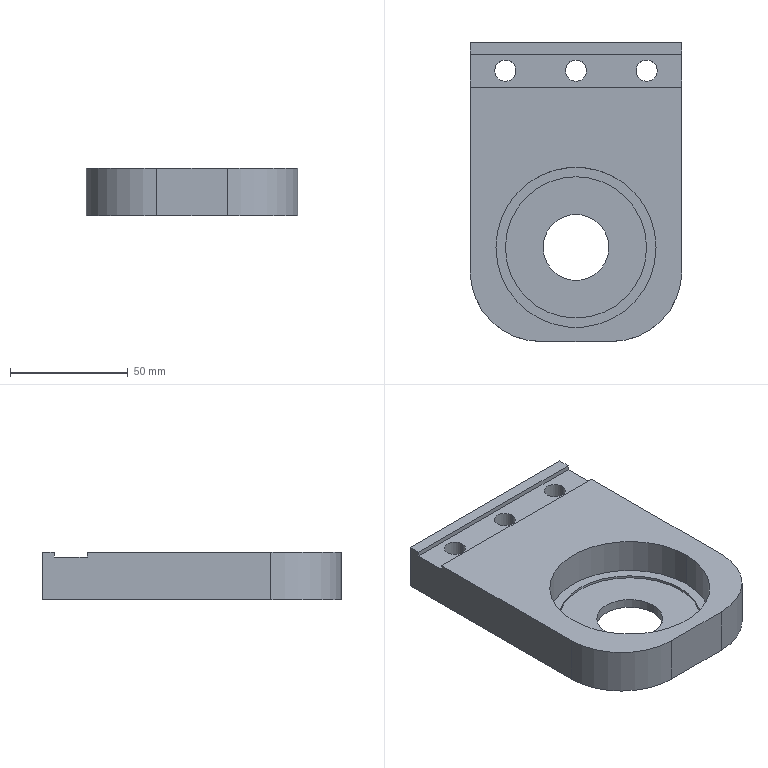Part | SolidWorks | features ICE 4, MoveFace 2, Extrusion 1, Fillet 1, HoleWzd 1 | 1 solid | 35 faces | box 90 x 127.02 x 20 mm | volume 152136 mm3 | cylinder 20 | plane 15 | commonest cylinder face diameters 9 x6 15 x6 60 x4 28 x2 68 x2
STEP:
#1=CARTESIAN_POINT('',(37.5,55.02,9.));
#2=VERTEX_POINT('',#1);
#3=CARTESIAN_POINT('',(22.5,55.02,9.));
#4=VERTEX_POINT('',#3);
#5=CARTESIAN_POINT('',(30.,55.02,9.));
#6=DIRECTION('',(0.,0.,-1.));
#7=DIRECTION('',(-1.,0.,0.));
#8=AXIS2_PLACEMENT_3D('',#5,#6,#7);
#9=CIRCLE('',#8,7.5);
#10=EDGE_CURVE('',#2,#4,#9,.T.);
#11=ORIENTED_EDGE('',*,*,#10,.F.);
#12=CARTESIAN_POINT('',(37.5,55.02,0.));
#13=VERTEX_POINT('',#12);
#14=CARTESIAN_POINT('',(37.5,55.02,0.));
#15=DIRECTION('',(0.,0.,-1.));
#16=VECTOR('',#15,1000.);
#17=LINE('',#14,#16);
#18=EDGE_CURVE('',#2,#13,#17,.T.);
#19=ORIENTED_EDGE('',*,*,#18,.T.);
#20=CARTESIAN_POINT('',(22.5,55.02,0.));
#21=VERTEX_POINT('',#20);
#22=CARTESIAN_POINT('',(30.,55.02,0.));
#23=DIRECTION('',(0.,0.,-1.));
#24=DIRECTION('',(-1.,0.,0.));
#25=AXIS2_PLACEMENT_3D('',#22,#23,#24);
#26=CIRCLE('',#25,7.5);
#27=EDGE_CURVE('',#13,#21,#26,.T.);
#28=ORIENTED_EDGE('',*,*,#27,.T.);
#29=CARTESIAN_POINT('',(22.5,55.02,0.));
#30=DIRECTION('',(0.,0.,-1.));
#31=VECTOR('',#30,1000.);
#32=LINE('',#29,#31);
#33=EDGE_CURVE('',#4,#21,#32,.T.);
#34=ORIENTED_EDGE('',*,*,#33,.F.);
#35=EDGE_LOOP('',(#11,#19,#28,#34));
#36=FACE_OUTER_BOUND('',#35,.T.);
#37=CARTESIAN_POINT('',(30.,55.02,0.));
#38=DIRECTION('',(0.,0.,-1.));
#39=DIRECTION('',(-1.,0.,0.));
#40=AXIS2_PLACEMENT_3D('',#37,#38,#39);
#41=CYLINDRICAL_SURFACE('',#40,7.5);
#42=ADVANCED_FACE('',(#36),#41,.F.);
#43=CARTESIAN_POINT('',(7.5,55.02,9.));
#44=VERTEX_POINT('',#43);
#45=CARTESIAN_POINT('',(-7.5,55.02,9.));
#46=VERTEX_POINT('',#45);
#47=CARTESIAN_POINT('',(0.,55.02,9.));
#48=DIRECTION('',(0.,0.,-1.));
#49=DIRECTION('',(-1.,0.,0.));
#50=AXIS2_PLACEMENT_3D('',#47,#48,#49);
#51=CIRCLE('',#50,7.5);
#52=EDGE_CURVE('',#44,#46,#51,.T.);
#53=ORIENTED_EDGE('',*,*,#52,.F.);
#54=CARTESIAN_POINT('',(7.5,55.02,0.));
#55=VERTEX_POINT('',#54);
#56=CARTESIAN_POINT('',(7.5,55.02,0.));
#57=DIRECTION('',(0.,0.,-1.));
#58=VECTOR('',#57,1000.);
#59=LINE('',#56,#58);
#60=EDGE_CURVE('',#44,#55,#59,.T.);
#61=ORIENTED_EDGE('',*,*,#60,.T.);
#62=CARTESIAN_POINT('',(-7.5,55.02,0.));
#63=VERTEX_POINT('',#62);
#64=CARTESIAN_POINT('',(0.,55.02,0.));
#65=DIRECTION('',(0.,0.,-1.));
#66=DIRECTION('',(-1.,0.,0.));
#67=AXIS2_PLACEMENT_3D('',#64,#65,#66);
#68=CIRCLE('',#67,7.5);
#69=EDGE_CURVE('',#55,#63,#68,.T.);
#70=ORIENTED_EDGE('',*,*,#69,.T.);
#71=CARTESIAN_POINT('',(-7.5,55.02,0.));
#72=DIRECTION('',(0.,0.,-1.));
#73=VECTOR('',#72,1000.);
#74=LINE('',#71,#73);
#75=EDGE_CURVE('',#46,#63,#74,.T.);
#76=ORIENTED_EDGE('',*,*,#75,.F.);
#77=EDGE_LOOP('',(#53,#61,#70,#76));
#78=FACE_OUTER_BOUND('',#77,.T.);
#79=CARTESIAN_POINT('',(0.,55.02,0.));
#80=DIRECTION('',(0.,0.,-1.));
#81=DIRECTION('',(-1.,0.,0.));
#82=AXIS2_PLACEMENT_3D('',#79,#80,#81);
#83=CYLINDRICAL_SURFACE('',#82,7.5);
#84=ADVANCED_FACE('',(#78),#83,.F.);
#85=CARTESIAN_POINT('',(-22.5,55.02,9.));
#86=VERTEX_POINT('',#85);
#87=CARTESIAN_POINT('',(-37.5,55.02,9.));
#88=VERTEX_POINT('',#87);
#89=CARTESIAN_POINT('',(-30.,55.02,9.));
#90=DIRECTION('',(0.,0.,-1.));
#91=DIRECTION('',(-1.,0.,0.));
#92=AXIS2_PLACEMENT_3D('',#89,#90,#91);
#93=CIRCLE('',#92,7.5);
#94=EDGE_CURVE('',#86,#88,#93,.T.);
#95=ORIENTED_EDGE('',*,*,#94,.F.);
#96=CARTESIAN_POINT('',(-22.5,55.02,0.));
#97=VERTEX_POINT('',#96);
#98=CARTESIAN_POINT('',(-22.5,55.02,0.));
#99=DIRECTION('',(0.,0.,-1.));
#100=VECTOR('',#99,1000.);
#101=LINE('',#98,#100);
#102=EDGE_CURVE('',#86,#97,#101,.T.);
#103=ORIENTED_EDGE('',*,*,#102,.T.);
#104=CARTESIAN_POINT('',(-37.5,55.02,0.));
#105=VERTEX_POINT('',#104);
#106=CARTESIAN_POINT('',(-30.,55.02,0.));
#107=DIRECTION('',(0.,0.,-1.));
#108=DIRECTION('',(-1.,0.,0.));
#109=AXIS2_PLACEMENT_3D('',#106,#107,#108);
#110=CIRCLE('',#109,7.5);
#111=EDGE_CURVE('',#97,#105,#110,.T.);
#112=ORIENTED_EDGE('',*,*,#111,.T.);
#113=CARTESIAN_POINT('',(-37.5,55.02,0.));
#114=DIRECTION('',(0.,0.,-1.));
#115=VECTOR('',#114,1000.);
#116=LINE('',#113,#115);
#117=EDGE_CURVE('',#88,#105,#116,.T.);
#118=ORIENTED_EDGE('',*,*,#117,.F.);
#119=EDGE_LOOP('',(#95,#103,#112,#118));
#120=FACE_OUTER_BOUND('',#119,.T.);
#121=CARTESIAN_POINT('',(-30.,55.02,0.));
#122=DIRECTION('',(0.,0.,-1.));
#123=DIRECTION('',(-1.,0.,0.));
#124=AXIS2_PLACEMENT_3D('',#121,#122,#123);
#125=CYLINDRICAL_SURFACE('',#124,7.5);
#126=ADVANCED_FACE('',(#120),#125,.F.);
#127=CARTESIAN_POINT('',(-14.,-20.,0.));
#128=VERTEX_POINT('',#127);
#129=CARTESIAN_POINT('',(14.,-20.,0.));
#130=VERTEX_POINT('',#129);
#131=CARTESIAN_POINT('',(0.,-20.,0.));
#132=DIRECTION('',(0.,0.,1.));
#133=DIRECTION('',(1.,0.,0.));
#134=AXIS2_PLACEMENT_3D('',#131,#132,#133);
#135=CIRCLE('',#134,14.);
#136=EDGE_CURVE('',#128,#130,#135,.T.);
#137=ORIENTED_EDGE('',*,*,#136,.F.);
#138=CARTESIAN_POINT('',(-14.,-20.,4.));
#139=VERTEX_POINT('',#138);
#140=CARTESIAN_POINT('',(-14.,-20.,-6.));
#141=DIRECTION('',(0.,0.,1.));
#142=VECTOR('',#141,1000.);
#143=LINE('',#140,#142);
#144=EDGE_CURVE('',#128,#139,#143,.T.);
#145=ORIENTED_EDGE('',*,*,#144,.T.);
#146=CARTESIAN_POINT('',(14.,-20.,4.));
#147=VERTEX_POINT('',#146);
#148=CARTESIAN_POINT('',(0.,-20.,4.));
#149=DIRECTION('',(0.,0.,1.));
#150=DIRECTION('',(1.,0.,0.));
#151=AXIS2_PLACEMENT_3D('',#148,#149,#150);
#152=CIRCLE('',#151,14.);
#153=EDGE_CURVE('',#139,#147,#152,.T.);
#154=ORIENTED_EDGE('',*,*,#153,.T.);
#155=CARTESIAN_POINT('',(14.,-20.,-6.));
#156=DIRECTION('',(0.,0.,1.));
#157=VECTOR('',#156,1000.);
#158=LINE('',#155,#157);
#159=EDGE_CURVE('',#130,#147,#158,.T.);
#160=ORIENTED_EDGE('',*,*,#159,.F.);
#161=EDGE_LOOP('',(#137,#145,#154,#160));
#162=FACE_OUTER_BOUND('',#161,.T.);
#163=CARTESIAN_POINT('',(0.,-20.,-6.));
#164=DIRECTION('',(0.,0.,1.));
#165=DIRECTION('',(1.,0.,0.));
#166=AXIS2_PLACEMENT_3D('',#163,#164,#165);
#167=CYLINDRICAL_SURFACE('',#166,14.);
#168=ADVANCED_FACE('',(#162),#167,.F.);
#169=CARTESIAN_POINT('',(-30.,-20.,4.));
#170=VERTEX_POINT('',#169);
#171=CARTESIAN_POINT('',(30.,-20.,4.));
#172=VERTEX_POINT('',#171);
#173=CARTESIAN_POINT('',(0.,-20.,4.));
#174=DIRECTION('',(0.,0.,1.));
#175=DIRECTION('',(1.,0.,0.));
#176=AXIS2_PLACEMENT_3D('',#173,#174,#175);
#177=CIRCLE('',#176,30.);
#178=EDGE_CURVE('',#170,#172,#177,.T.);
#179=ORIENTED_EDGE('',*,*,#178,.F.);
#180=CARTESIAN_POINT('',(-30.,-20.,5.));
#181=VERTEX_POINT('',#180);
#182=CARTESIAN_POINT('',(-30.,-20.,4.));
#183=DIRECTION('',(0.,0.,1.));
#184=VECTOR('',#183,1000.);
#185=LINE('',#182,#184);
#186=EDGE_CURVE('',#170,#181,#185,.T.);
#187=ORIENTED_EDGE('',*,*,#186,.T.);
#188=CARTESIAN_POINT('',(30.,-20.,5.));
#189=VERTEX_POINT('',#188);
#190=CARTESIAN_POINT('',(0.,-20.,5.));
#191=DIRECTION('',(0.,0.,1.));
#192=DIRECTION('',(1.,0.,0.));
#193=AXIS2_PLACEMENT_3D('',#190,#191,#192);
#194=CIRCLE('',#193,30.);
#195=EDGE_CURVE('',#181,#189,#194,.T.);
#196=ORIENTED_EDGE('',*,*,#195,.T.);
#197=CARTESIAN_POINT('',(30.,-20.,4.));
#198=DIRECTION('',(0.,0.,1.));
#199=VECTOR('',#198,1000.);
#200=LINE('',#197,#199);
#201=EDGE_CURVE('',#172,#189,#200,.T.);
#202=ORIENTED_EDGE('',*,*,#201,.F.);
#203=EDGE_LOOP('',(#179,#187,#196,#202));
#204=FACE_OUTER_BOUND('',#203,.T.);
#205=CARTESIAN_POINT('',(0.,-20.,4.));
#206=DIRECTION('',(0.,0.,1.));
#207=DIRECTION('',(1.,0.,0.));
#208=AXIS2_PLACEMENT_3D('',#205,#206,#207);
#209=CYLINDRICAL_SURFACE('',#208,30.);
#210=ADVANCED_FACE('',(#204),#209,.F.);
#211=CARTESIAN_POINT('',(-34.,-20.,5.));
#212=VERTEX_POINT('',#211);
#213=CARTESIAN_POINT('',(34.,-20.,5.));
#214=VERTEX_POINT('',#213);
#215=CARTESIAN_POINT('',(0.,-20.,5.));
#216=DIRECTION('',(0.,0.,1.));
#217=DIRECTION('',(1.,0.,0.));
#218=AXIS2_PLACEMENT_3D('',#215,#216,#217);
#219=CIRCLE('',#218,34.);
#220=EDGE_CURVE('',#212,#214,#219,.T.);
#221=ORIENTED_EDGE('',*,*,#220,.F.);
#222=CARTESIAN_POINT('',(-34.,-20.,20.));
#223=VERTEX_POINT('',#222);
#224=CARTESIAN_POINT('',(-34.,-20.,5.));
#225=DIRECTION('',(0.,0.,1.));
#226=VECTOR('',#225,1000.);
#227=LINE('',#224,#226);
#228=EDGE_CURVE('',#212,#223,#227,.T.);
#229=ORIENTED_EDGE('',*,*,#228,.T.);
#230=CARTESIAN_POINT('',(34.,-20.,20.));
#231=VERTEX_POINT('',#230);
#232=CARTESIAN_POINT('',(0.,-20.,20.));
#233=DIRECTION('',(0.,0.,1.));
#234=DIRECTION('',(1.,0.,0.));
#235=AXIS2_PLACEMENT_3D('',#232,#233,#234);
#236=CIRCLE('',#235,34.);
#237=EDGE_CURVE('',#223,#231,#236,.T.);
#238=ORIENTED_EDGE('',*,*,#237,.T.);
#239=CARTESIAN_POINT('',(34.,-20.,5.));
#240=DIRECTION('',(0.,0.,1.));
#241=VECTOR('',#240,1000.);
#242=LINE('',#239,#241);
#243=EDGE_CURVE('',#214,#231,#242,.T.);
#244=ORIENTED_EDGE('',*,*,#243,.F.);
#245=EDGE_LOOP('',(#221,#229,#238,#244));
#246=FACE_OUTER_BOUND('',#245,.T.);
#247=CARTESIAN_POINT('',(0.,-20.,5.));
#248=DIRECTION('',(0.,0.,1.));
#249=DIRECTION('',(1.,0.,0.));
#250=AXIS2_PLACEMENT_3D('',#247,#248,#249);
#251=CYLINDRICAL_SURFACE('',#250,34.);
#252=ADVANCED_FACE('',(#246),#251,.F.);
#253=CARTESIAN_POINT('',(34.5,55.02,18.));
#254=VERTEX_POINT('',#253);
#255=CARTESIAN_POINT('',(25.5,55.02,18.));
#256=VERTEX_POINT('',#255);
#257=CARTESIAN_POINT('',(30.,55.02,18.));
#258=DIRECTION('',(0.,0.,-1.));
#259=DIRECTION('',(1.,0.,0.));
#260=AXIS2_PLACEMENT_3D('',#257,#258,#259);
#261=CIRCLE('',#260,4.5);
#262=EDGE_CURVE('',#254,#256,#261,.T.);
#263=ORIENTED_EDGE('',*,*,#262,.F.);
#264=CARTESIAN_POINT('',(34.5,55.02,9.));
#265=VERTEX_POINT('',#264);
#266=CARTESIAN_POINT('',(34.5,55.02,0.));
#267=DIRECTION('',(0.,0.,-1.));
#268=VECTOR('',#267,1000.);
#269=LINE('',#266,#268);
#270=EDGE_CURVE('',#254,#265,#269,.T.);
#271=ORIENTED_EDGE('',*,*,#270,.T.);
#272=CARTESIAN_POINT('',(25.5,55.02,9.));
#273=VERTEX_POINT('',#272);
#274=CARTESIAN_POINT('',(30.,55.02,9.));
#275=DIRECTION('',(0.,0.,-1.));
#276=DIRECTION('',(-1.,0.,0.));
#277=AXIS2_PLACEMENT_3D('',#274,#275,#276);
#278=CIRCLE('',#277,4.5);
#279=EDGE_CURVE('',#265,#273,#278,.T.);
#280=ORIENTED_EDGE('',*,*,#279,.T.);
#281=CARTESIAN_POINT('',(25.5,55.02,0.));
#282=DIRECTION('',(0.,0.,-1.));
#283=VECTOR('',#282,1000.);
#284=LINE('',#281,#283);
#285=EDGE_CURVE('',#256,#273,#284,.T.);
#286=ORIENTED_EDGE('',*,*,#285,.F.);
#287=EDGE_LOOP('',(#263,#271,#280,#286));
#288=FACE_OUTER_BOUND('',#287,.T.);
#289=CARTESIAN_POINT('',(30.,55.02,0.));
#290=DIRECTION('',(0.,0.,-1.));
#291=DIRECTION('',(-1.,0.,0.));
#292=AXIS2_PLACEMENT_3D('',#289,#290,#291);
#293=CYLINDRICAL_SURFACE('',#292,4.5);
#294=ADVANCED_FACE('',(#288),#293,.F.);
#295=CARTESIAN_POINT('',(4.5,55.02,18.));
#296=VERTEX_POINT('',#295);
#297=CARTESIAN_POINT('',(-4.5,55.02,18.));
#298=VERTEX_POINT('',#297);
#299=CARTESIAN_POINT('',(0.,55.02,18.));
#300=DIRECTION('',(0.,0.,-1.));
#301=DIRECTION('',(1.,0.,0.));
#302=AXIS2_PLACEMENT_3D('',#299,#300,#301);
#303=CIRCLE('',#302,4.5);
#304=EDGE_CURVE('',#296,#298,#303,.T.);
#305=ORIENTED_EDGE('',*,*,#304,.F.);
#306=CARTESIAN_POINT('',(4.5,55.02,9.));
#307=VERTEX_POINT('',#306);
#308=CARTESIAN_POINT('',(4.5,55.02,0.));
#309=DIRECTION('',(0.,0.,-1.));
#310=VECTOR('',#309,1000.);
#311=LINE('',#308,#310);
#312=EDGE_CURVE('',#296,#307,#311,.T.);
#313=ORIENTED_EDGE('',*,*,#312,.T.);
#314=CARTESIAN_POINT('',(-4.5,55.02,9.));
#315=VERTEX_POINT('',#314);
#316=CARTESIAN_POINT('',(0.,55.02,9.));
#317=DIRECTION('',(0.,0.,-1.));
#318=DIRECTION('',(-1.,0.,0.));
#319=AXIS2_PLACEMENT_3D('',#316,#317,#318);
#320=CIRCLE('',#319,4.5);
#321=EDGE_CURVE('',#307,#315,#320,.T.);
#322=ORIENTED_EDGE('',*,*,#321,.T.);
#323=CARTESIAN_POINT('',(-4.5,55.02,0.));
#324=DIRECTION('',(0.,0.,-1.));
#325=VECTOR('',#324,1000.);
#326=LINE('',#323,#325);
#327=EDGE_CURVE('',#298,#315,#326,.T.);
#328=ORIENTED_EDGE('',*,*,#327,.F.);
#329=EDGE_LOOP('',(#305,#313,#322,#328));
#330=FACE_OUTER_BOUND('',#329,.T.);
#331=CARTESIAN_POINT('',(0.,55.02,0.));
#332=DIRECTION('',(0.,0.,-1.));
#333=DIRECTION('',(-1.,0.,0.));
#334=AXIS2_PLACEMENT_3D('',#331,#332,#333);
#335=CYLINDRICAL_SURFACE('',#334,4.5);
#336=ADVANCED_FACE('',(#330),#335,.F.);
#337=CARTESIAN_POINT('',(-25.5,55.02,18.));
#338=VERTEX_POINT('',#337);
#339=CARTESIAN_POINT('',(-34.5,55.02,18.));
#340=VERTEX_POINT('',#339);
#341=CARTESIAN_POINT('',(-30.,55.02,18.));
#342=DIRECTION('',(0.,0.,-1.));
#343=DIRECTION('',(1.,0.,0.));
#344=AXIS2_PLACEMENT_3D('',#341,#342,#343);
#345=CIRCLE('',#344,4.5);
#346=EDGE_CURVE('',#338,#340,#345,.T.);
#347=ORIENTED_EDGE('',*,*,#346,.F.);
#348=CARTESIAN_POINT('',(-25.5,55.02,9.));
#349=VERTEX_POINT('',#348);
#350=CARTESIAN_POINT('',(-25.5,55.02,0.));
#351=DIRECTION('',(0.,0.,-1.));
#352=VECTOR('',#351,1000.);
#353=LINE('',#350,#352);
#354=EDGE_CURVE('',#338,#349,#353,.T.);
#355=ORIENTED_EDGE('',*,*,#354,.T.);
#356=CARTESIAN_POINT('',(-34.5,55.02,9.));
#357=VERTEX_POINT('',#356);
#358=CARTESIAN_POINT('',(-30.,55.02,9.));
#359=DIRECTION('',(0.,0.,-1.));
#360=DIRECTION('',(-1.,0.,0.));
#361=AXIS2_PLACEMENT_3D('',#358,#359,#360);
#362=CIRCLE('',#361,4.5);
#363=EDGE_CURVE('',#349,#357,#362,.T.);
#364=ORIENTED_EDGE('',*,*,#363,.T.);
#365=CARTESIAN_POINT('',(-34.5,55.02,0.));
#366=DIRECTION('',(0.,0.,-1.));
#367=VECTOR('',#366,1000.);
#368=LINE('',#365,#367);
#369=EDGE_CURVE('',#340,#357,#368,.T.);
#370=ORIENTED_EDGE('',*,*,#369,.F.);
#371=EDGE_LOOP('',(#347,#355,#364,#370));
#372=FACE_OUTER_BOUND('',#371,.T.);
#373=CARTESIAN_POINT('',(-30.,55.02,0.));
#374=DIRECTION('',(0.,0.,-1.));
#375=DIRECTION('',(-1.,0.,0.));
#376=AXIS2_PLACEMENT_3D('',#373,#374,#375);
#377=CYLINDRICAL_SURFACE('',#376,4.5);
#378=ADVANCED_FACE('',(#372),#377,.F.);
#379=CARTESIAN_POINT('',(45.,62.02,20.));
#380=VERTEX_POINT('',#379);
#381=CARTESIAN_POINT('',(-45.,62.02,20.));
#382=VERTEX_POINT('',#381);
#383=CARTESIAN_POINT('',(-45.,62.02,20.));
#384=DIRECTION('',(-1.,0.,0.));
#385=VECTOR('',#384,1000.);
#386=LINE('',#383,#385);
#387=EDGE_CURVE('',#380,#382,#386,.T.);
#388=ORIENTED_EDGE('',*,*,#387,.F.);
#389=CARTESIAN_POINT('',(45.,67.02,20.));
#390=VERTEX_POINT('',#389);
#391=CARTESIAN_POINT('',(45.,60.,20.));
#392=DIRECTION('',(0.,1.,0.));
#393=VECTOR('',#392,1000.);
#394=LINE('',#391,#393);
#395=EDGE_CURVE('',#380,#390,#394,.T.);
#396=ORIENTED_EDGE('',*,*,#395,.T.);
#397=CARTESIAN_POINT('',(-45.,67.02,20.));
#398=VERTEX_POINT('',#397);
#399=CARTESIAN_POINT('',(-45.,67.02,20.));
#400=DIRECTION('',(-1.,0.,0.));
#401=VECTOR('',#400,1000.);
#402=LINE('',#399,#401);
#403=EDGE_CURVE('',#390,#398,#402,.T.);
#404=ORIENTED_EDGE('',*,*,#403,.T.);
#405=CARTESIAN_POINT('',(-45.,60.,20.));
#406=DIRECTION('',(0.,-1.,0.));
#407=VECTOR('',#406,1000.);
#408=LINE('',#405,#407);
#409=EDGE_CURVE('',#398,#382,#408,.T.);
#410=ORIENTED_EDGE('',*,*,#409,.T.);
#411=EDGE_LOOP('',(#388,#396,#404,#410));
#412=FACE_OUTER_BOUND('',#411,.T.);
#413=CARTESIAN_POINT('',(0.,0.,20.));
#414=DIRECTION('',(0.,0.,1.));
#415=DIRECTION('',(1.,0.,0.));
#416=AXIS2_PLACEMENT_3D('',#413,#414,#415);
#417=PLANE('',#416);
#418=ADVANCED_FACE('',(#412),#417,.T.);
#419=ORIENTED_EDGE('',*,*,#354,.F.);
#420=CARTESIAN_POINT('',(-30.,55.02,18.));
#421=DIRECTION('',(0.,0.,-1.));
#422=DIRECTION('',(1.,0.,0.));
#423=AXIS2_PLACEMENT_3D('',#420,#421,#422);
#424=CIRCLE('',#423,4.5);
#425=EDGE_CURVE('',#340,#338,#424,.T.);
#426=ORIENTED_EDGE('',*,*,#425,.F.);
#427=ORIENTED_EDGE('',*,*,#369,.T.);
#428=CARTESIAN_POINT('',(-30.,55.02,9.));
#429=DIRECTION('',(0.,0.,-1.));
#430=DIRECTION('',(-1.,0.,0.));
#431=AXIS2_PLACEMENT_3D('',#428,#429,#430);
#432=CIRCLE('',#431,4.5);
#433=EDGE_CURVE('',#357,#349,#432,.T.);
#434=ORIENTED_EDGE('',*,*,#433,.T.);
#435=EDGE_LOOP('',(#419,#426,#427,#434));
#436=FACE_OUTER_BOUND('',#435,.T.);
#437=CARTESIAN_POINT('',(-30.,55.02,0.));
#438=DIRECTION('',(0.,0.,-1.));
#439=DIRECTION('',(-1.,0.,0.));
#440=AXIS2_PLACEMENT_3D('',#437,#438,#439);
#441=CYLINDRICAL_SURFACE('',#440,4.5);
#442=ADVANCED_FACE('',(#436),#441,.F.);
#443=ORIENTED_EDGE('',*,*,#312,.F.);
#444=CARTESIAN_POINT('',(0.,55.02,18.));
#445=DIRECTION('',(0.,0.,-1.));
#446=DIRECTION('',(1.,0.,0.));
#447=AXIS2_PLACEMENT_3D('',#444,#445,#446);
#448=CIRCLE('',#447,4.5);
#449=EDGE_CURVE('',#298,#296,#448,.T.);
#450=ORIENTED_EDGE('',*,*,#449,.F.);
#451=ORIENTED_EDGE('',*,*,#327,.T.);
#452=CARTESIAN_POINT('',(0.,55.02,9.));
#453=DIRECTION('',(0.,0.,-1.));
#454=DIRECTION('',(-1.,0.,0.));
#455=AXIS2_PLACEMENT_3D('',#452,#453,#454);
#456=CIRCLE('',#455,4.5);
#457=EDGE_CURVE('',#315,#307,#456,.T.);
#458=ORIENTED_EDGE('',*,*,#457,.T.);
#459=EDGE_LOOP('',(#443,#450,#451,#458));
#460=FACE_OUTER_BOUND('',#459,.T.);
#461=CARTESIAN_POINT('',(0.,55.02,0.));
#462=DIRECTION('',(0.,0.,-1.));
#463=DIRECTION('',(-1.,0.,0.));
#464=AXIS2_PLACEMENT_3D('',#461,#462,#463);
#465=CYLINDRICAL_SURFACE('',#464,4.5);
#466=ADVANCED_FACE('',(#460),#465,.F.);
#467=ORIENTED_EDGE('',*,*,#270,.F.);
#468=CARTESIAN_POINT('',(30.,55.02,18.));
#469=DIRECTION('',(0.,0.,-1.));
#470=DIRECTION('',(1.,0.,0.));
#471=AXIS2_PLACEMENT_3D('',#468,#469,#470);
#472=CIRCLE('',#471,4.5);
#473=EDGE_CURVE('',#256,#254,#472,.T.);
#474=ORIENTED_EDGE('',*,*,#473,.F.);
#475=ORIENTED_EDGE('',*,*,#285,.T.);
#476=CARTESIAN_POINT('',(30.,55.02,9.));
#477=DIRECTION('',(0.,0.,-1.));
#478=DIRECTION('',(-1.,0.,0.));
#479=AXIS2_PLACEMENT_3D('',#476,#477,#478);
#480=CIRCLE('',#479,4.5);
#481=EDGE_CURVE('',#273,#265,#480,.T.);
#482=ORIENTED_EDGE('',*,*,#481,.T.);
#483=EDGE_LOOP('',(#467,#474,#475,#482));
#484=FACE_OUTER_BOUND('',#483,.T.);
#485=CARTESIAN_POINT('',(30.,55.02,0.));
#486=DIRECTION('',(0.,0.,-1.));
#487=DIRECTION('',(-1.,0.,0.));
#488=AXIS2_PLACEMENT_3D('',#485,#486,#487);
#489=CYLINDRICAL_SURFACE('',#488,4.5);
#490=ADVANCED_FACE('',(#484),#489,.F.);
#491=ORIENTED_EDGE('',*,*,#395,.F.);
#492=CARTESIAN_POINT('',(45.,62.02,18.));
#493=VERTEX_POINT('',#492);
#494=CARTESIAN_POINT('',(45.,62.02,18.));
#495=DIRECTION('',(0.,0.,1.));
#496=VECTOR('',#495,1000.);
#497=LINE('',#494,#496);
#498=EDGE_CURVE('',#493,#380,#497,.T.);
#499=ORIENTED_EDGE('',*,*,#498,.F.);
#500=CARTESIAN_POINT('',(45.,48.02,18.));
#501=VERTEX_POINT('',#500);
#502=CARTESIAN_POINT('',(45.,62.02,18.));
#503=DIRECTION('',(0.,1.,0.));
#504=VECTOR('',#503,1000.);
#505=LINE('',#502,#504);
#506=EDGE_CURVE('',#501,#493,#505,.T.);
#507=ORIENTED_EDGE('',*,*,#506,.F.);
#508=CARTESIAN_POINT('',(45.,48.02,20.));
#509=VERTEX_POINT('',#508);
#510=CARTESIAN_POINT('',(45.,48.02,18.));
#511=DIRECTION('',(0.,0.,1.));
#512=VECTOR('',#511,1000.);
#513=LINE('',#510,#512);
#514=EDGE_CURVE('',#501,#509,#513,.T.);
#515=ORIENTED_EDGE('',*,*,#514,.T.);
#516=CARTESIAN_POINT('',(45.,-30.,20.));
#517=VERTEX_POINT('',#516);
#518=CARTESIAN_POINT('',(45.,60.,20.));
#519=DIRECTION('',(0.,1.,0.));
#520=VECTOR('',#519,1000.);
#521=LINE('',#518,#520);
#522=EDGE_CURVE('',#517,#509,#521,.T.);
#523=ORIENTED_EDGE('',*,*,#522,.F.);
#524=CARTESIAN_POINT('',(45.,-30.,0.));
#525=VERTEX_POINT('',#524);
#526=CARTESIAN_POINT('',(45.,-30.,20.));
#527=DIRECTION('',(0.,0.,-1.));
#528=VECTOR('',#527,1000.);
#529=LINE('',#526,#528);
#530=EDGE_CURVE('',#517,#525,#529,.T.);
#531=ORIENTED_EDGE('',*,*,#530,.T.);
#532=CARTESIAN_POINT('',(45.,67.02,0.));
#533=VERTEX_POINT('',#532);
#534=CARTESIAN_POINT('',(45.,60.,0.));
#535=DIRECTION('',(0.,1.,0.));
#536=VECTOR('',#535,1000.);
#537=LINE('',#534,#536);
#538=EDGE_CURVE('',#525,#533,#537,.T.);
#539=ORIENTED_EDGE('',*,*,#538,.T.);
#540=CARTESIAN_POINT('',(45.,67.02,20.));
#541=DIRECTION('',(0.,0.,-1.));
#542=VECTOR('',#541,1000.);
#543=LINE('',#540,#542);
#544=EDGE_CURVE('',#390,#533,#543,.T.);
#545=ORIENTED_EDGE('',*,*,#544,.F.);
#546=EDGE_LOOP('',(#491,#499,#507,#515,#523,#531,#539,#545));
#547=FACE_OUTER_BOUND('',#546,.T.);
#548=CARTESIAN_POINT('',(45.,60.,20.));
#549=DIRECTION('',(-1.,0.,0.));
#550=DIRECTION('',(0.,-1.,0.));
#551=AXIS2_PLACEMENT_3D('',#548,#549,#550);
#552=PLANE('',#551);
#553=ADVANCED_FACE('',(#547),#552,.F.);
#554=CARTESIAN_POINT('',(-45.,67.02,0.));
#555=VERTEX_POINT('',#554);
#556=CARTESIAN_POINT('',(-45.,67.02,0.));
#557=DIRECTION('',(-1.,0.,0.));
#558=VECTOR('',#557,1000.);
#559=LINE('',#556,#558);
#560=EDGE_CURVE('',#533,#555,#559,.T.);
#561=ORIENTED_EDGE('',*,*,#560,.T.);
#562=CARTESIAN_POINT('',(-45.,67.02,20.));
#563=DIRECTION('',(0.,0.,-1.));
#564=VECTOR('',#563,1000.);
#565=LINE('',#562,#564);
#566=EDGE_CURVE('',#398,#555,#565,.T.);
#567=ORIENTED_EDGE('',*,*,#566,.F.);
#568=ORIENTED_EDGE('',*,*,#403,.F.);
#569=ORIENTED_EDGE('',*,*,#544,.T.);
#570=EDGE_LOOP('',(#561,#567,#568,#569));
#571=FACE_OUTER_BOUND('',#570,.T.);
#572=CARTESIAN_POINT('',(-45.,67.02,20.));
#573=DIRECTION('',(0.,-1.,0.));
#574=DIRECTION('',(0.,0.,-1.));
#575=AXIS2_PLACEMENT_3D('',#572,#573,#574);
#576=PLANE('',#575);
#577=ADVANCED_FACE('',(#571),#576,.F.);
#578=CARTESIAN_POINT('',(-45.,62.02,18.));
#579=VERTEX_POINT('',#578);
#580=CARTESIAN_POINT('',(-45.,48.02,18.));
#581=VERTEX_POINT('',#580);
#582=CARTESIAN_POINT('',(-45.,62.02,18.));
#583=DIRECTION('',(0.,-1.,0.));
#584=VECTOR('',#583,1000.);
#585=LINE('',#582,#584);
#586=EDGE_CURVE('',#579,#581,#585,.T.);
#587=ORIENTED_EDGE('',*,*,#586,.F.);
#588=CARTESIAN_POINT('',(-45.,62.02,18.));
#589=DIRECTION('',(0.,0.,1.));
#590=VECTOR('',#589,1000.);
#591=LINE('',#588,#590);
#592=EDGE_CURVE('',#579,#382,#591,.T.);
#593=ORIENTED_EDGE('',*,*,#592,.T.);
#594=ORIENTED_EDGE('',*,*,#409,.F.);
#595=ORIENTED_EDGE('',*,*,#566,.T.);
#596=CARTESIAN_POINT('',(-45.,-30.,0.));
#597=VERTEX_POINT('',#596);
#598=CARTESIAN_POINT('',(-45.,60.,0.));
#599=DIRECTION('',(0.,-1.,0.));
#600=VECTOR('',#599,1000.);
#601=LINE('',#598,#600);
#602=EDGE_CURVE('',#555,#597,#601,.T.);
#603=ORIENTED_EDGE('',*,*,#602,.T.);
#604=CARTESIAN_POINT('',(-45.,-30.,20.));
#605=VERTEX_POINT('',#604);
#606=CARTESIAN_POINT('',(-45.,-30.,20.));
#607=DIRECTION('',(0.,0.,1.));
#608=VECTOR('',#607,1000.);
#609=LINE('',#606,#608);
#610=EDGE_CURVE('',#597,#605,#609,.T.);
#611=ORIENTED_EDGE('',*,*,#610,.T.);
#612=CARTESIAN_POINT('',(-45.,48.02,20.));
#613=VERTEX_POINT('',#612);
#614=CARTESIAN_POINT('',(-45.,60.,20.));
#615=DIRECTION('',(0.,-1.,0.));
#616=VECTOR('',#615,1000.);
#617=LINE('',#614,#616);
#618=EDGE_CURVE('',#613,#605,#617,.T.);
#619=ORIENTED_EDGE('',*,*,#618,.F.);
#620=CARTESIAN_POINT('',(-45.,48.02,18.));
#621=DIRECTION('',(0.,0.,1.));
#622=VECTOR('',#621,1000.);
#623=LINE('',#620,#622);
#624=EDGE_CURVE('',#581,#613,#623,.T.);
#625=ORIENTED_EDGE('',*,*,#624,.F.);
#626=EDGE_LOOP('',(#587,#593,#594,#595,#603,#611,#619,#625));
#627=FACE_OUTER_BOUND('',#626,.T.);
#628=CARTESIAN_POINT('',(-45.,60.,20.));
#629=DIRECTION('',(1.,0.,0.));
#630=DIRECTION('',(0.,1.,0.));
#631=AXIS2_PLACEMENT_3D('',#628,#629,#630);
#632=PLANE('',#631);
#633=ADVANCED_FACE('',(#627),#632,.F.);
#634=CARTESIAN_POINT('',(-15.,-60.,0.));
#635=VERTEX_POINT('',#634);
#636=CARTESIAN_POINT('',(15.,-60.,0.));
#637=VERTEX_POINT('',#636);
#638=CARTESIAN_POINT('',(-45.,-60.,0.));
#639=DIRECTION('',(1.,0.,0.));
#640=VECTOR('',#639,1000.);
#641=LINE('',#638,#640);
#642=EDGE_CURVE('',#635,#637,#641,.T.);
#643=ORIENTED_EDGE('',*,*,#642,.T.);
#644=CARTESIAN_POINT('',(15.,-60.,20.));
#645=VERTEX_POINT('',#644);
#646=CARTESIAN_POINT('',(15.,-60.,20.));
#647=DIRECTION('',(0.,0.,1.));
#648=VECTOR('',#647,1000.);
#649=LINE('',#646,#648);
#650=EDGE_CURVE('',#637,#645,#649,.T.);
#651=ORIENTED_EDGE('',*,*,#650,.T.);
#652=CARTESIAN_POINT('',(-15.,-60.,20.));
#653=VERTEX_POINT('',#652);
#654=CARTESIAN_POINT('',(-45.,-60.,20.));
#655=DIRECTION('',(1.,0.,0.));
#656=VECTOR('',#655,1000.);
#657=LINE('',#654,#656);
#658=EDGE_CURVE('',#653,#645,#657,.T.);
#659=ORIENTED_EDGE('',*,*,#658,.F.);
#660=CARTESIAN_POINT('',(-15.,-60.,20.));
#661=DIRECTION('',(0.,0.,-1.));
#662=VECTOR('',#661,1000.);
#663=LINE('',#660,#662);
#664=EDGE_CURVE('',#653,#635,#663,.T.);
#665=ORIENTED_EDGE('',*,*,#664,.T.);
#666=EDGE_LOOP('',(#643,#651,#659,#665));
#667=FACE_OUTER_BOUND('',#666,.T.);
#668=CARTESIAN_POINT('',(-45.,-60.,20.));
#669=DIRECTION('',(0.,1.,0.));
#670=DIRECTION('',(0.,0.,1.));
#671=AXIS2_PLACEMENT_3D('',#668,#669,#670);
#672=PLANE('',#671);
#673=ADVANCED_FACE('',(#667),#672,.F.);
#674=CARTESIAN_POINT('',(-45.,48.02,20.));
#675=DIRECTION('',(1.,0.,0.));
#676=VECTOR('',#675,1000.);
#677=LINE('',#674,#676);
#678=EDGE_CURVE('',#613,#509,#677,.T.);
#679=ORIENTED_EDGE('',*,*,#678,.F.);
#680=ORIENTED_EDGE('',*,*,#618,.T.);
#681=CARTESIAN_POINT('',(-15.,-30.,20.));
#682=DIRECTION('',(0.,0.,1.));
#683=DIRECTION('',(1.,0.,0.));
#684=AXIS2_PLACEMENT_3D('',#681,#682,#683);
#685=CIRCLE('',#684,30.);
#686=EDGE_CURVE('',#605,#653,#685,.T.);
#687=ORIENTED_EDGE('',*,*,#686,.T.);
#688=ORIENTED_EDGE('',*,*,#658,.T.);
#689=CARTESIAN_POINT('',(15.,-30.,20.));
#690=DIRECTION('',(0.,0.,1.));
#691=DIRECTION('',(1.,0.,0.));
#692=AXIS2_PLACEMENT_3D('',#689,#690,#691);
#693=CIRCLE('',#692,30.);
#694=EDGE_CURVE('',#645,#517,#693,.T.);
#695=ORIENTED_EDGE('',*,*,#694,.T.);
#696=ORIENTED_EDGE('',*,*,#522,.T.);
#697=EDGE_LOOP('',(#679,#680,#687,#688,#695,#696));
#698=FACE_OUTER_BOUND('',#697,.T.);
#699=CARTESIAN_POINT('',(0.,-20.,20.));
#700=DIRECTION('',(0.,0.,1.));
#701=DIRECTION('',(1.,0.,0.));
#702=AXIS2_PLACEMENT_3D('',#699,#700,#701);
#703=CIRCLE('',#702,34.);
#704=EDGE_CURVE('',#231,#223,#703,.T.);
#705=ORIENTED_EDGE('',*,*,#704,.F.);
#706=ORIENTED_EDGE('',*,*,#237,.F.);
#707=EDGE_LOOP('',(#705,#706));
#708=FACE_BOUND('',#707,.T.);
#709=CARTESIAN_POINT('',(0.,0.,20.));
#710=DIRECTION('',(0.,0.,1.));
#711=DIRECTION('',(1.,0.,0.));
#712=AXIS2_PLACEMENT_3D('',#709,#710,#711);
#713=PLANE('',#712);
#714=ADVANCED_FACE('',(#698,#708),#713,.T.);
#715=CARTESIAN_POINT('',(30.,55.02,0.));
#716=DIRECTION('',(0.,0.,-1.));
#717=DIRECTION('',(-1.,0.,0.));
#718=AXIS2_PLACEMENT_3D('',#715,#716,#717);
#719=CIRCLE('',#718,7.5);
#720=EDGE_CURVE('',#21,#13,#719,.T.);
#721=ORIENTED_EDGE('',*,*,#720,.F.);
#722=ORIENTED_EDGE('',*,*,#27,.F.);
#723=EDGE_LOOP('',(#721,#722));
#724=FACE_BOUND('',#723,.T.);
#725=CARTESIAN_POINT('',(0.,55.02,0.));
#726=DIRECTION('',(0.,0.,-1.));
#727=DIRECTION('',(-1.,0.,0.));
#728=AXIS2_PLACEMENT_3D('',#725,#726,#727);
#729=CIRCLE('',#728,7.5);
#730=EDGE_CURVE('',#63,#55,#729,.T.);
#731=ORIENTED_EDGE('',*,*,#730,.F.);
#732=ORIENTED_EDGE('',*,*,#69,.F.);
#733=EDGE_LOOP('',(#731,#732));
#734=FACE_BOUND('',#733,.T.);
#735=CARTESIAN_POINT('',(-30.,55.02,0.));
#736=DIRECTION('',(0.,0.,-1.));
#737=DIRECTION('',(-1.,0.,0.));
#738=AXIS2_PLACEMENT_3D('',#735,#736,#737);
#739=CIRCLE('',#738,7.5);
#740=EDGE_CURVE('',#105,#97,#739,.T.);
#741=ORIENTED_EDGE('',*,*,#740,.F.);
#742=ORIENTED_EDGE('',*,*,#111,.F.);
#743=EDGE_LOOP('',(#741,#742));
#744=FACE_BOUND('',#743,.T.);
#745=CARTESIAN_POINT('',(0.,-20.,0.));
#746=DIRECTION('',(0.,0.,1.));
#747=DIRECTION('',(1.,0.,0.));
#748=AXIS2_PLACEMENT_3D('',#745,#746,#747);
#749=CIRCLE('',#748,14.);
#750=EDGE_CURVE('',#130,#128,#749,.T.);
#751=ORIENTED_EDGE('',*,*,#750,.T.);
#752=ORIENTED_EDGE('',*,*,#136,.T.);
#753=EDGE_LOOP('',(#751,#752));
#754=FACE_BOUND('',#753,.T.);
#755=ORIENTED_EDGE('',*,*,#538,.F.);
#756=CARTESIAN_POINT('',(15.,-30.,0.));
#757=DIRECTION('',(0.,0.,-1.));
#758=DIRECTION('',(1.,0.,0.));
#759=AXIS2_PLACEMENT_3D('',#756,#757,#758);
#760=CIRCLE('',#759,30.);
#761=EDGE_CURVE('',#525,#637,#760,.T.);
#762=ORIENTED_EDGE('',*,*,#761,.T.);
#763=ORIENTED_EDGE('',*,*,#642,.F.);
#764=CARTESIAN_POINT('',(-15.,-30.,0.));
#765=DIRECTION('',(0.,0.,-1.));
#766=DIRECTION('',(1.,0.,0.));
#767=AXIS2_PLACEMENT_3D('',#764,#765,#766);
#768=CIRCLE('',#767,30.);
#769=EDGE_CURVE('',#635,#597,#768,.T.);
#770=ORIENTED_EDGE('',*,*,#769,.T.);
#771=ORIENTED_EDGE('',*,*,#602,.F.);
#772=ORIENTED_EDGE('',*,*,#560,.F.);
#773=EDGE_LOOP('',(#755,#762,#763,#770,#771,#772));
#774=FACE_OUTER_BOUND('',#773,.T.);
#775=CARTESIAN_POINT('',(0.,0.,0.));
#776=DIRECTION('',(0.,0.,1.));
#777=DIRECTION('',(1.,0.,0.));
#778=AXIS2_PLACEMENT_3D('',#775,#776,#777);
#779=PLANE('',#778);
#780=ADVANCED_FACE('',(#724,#734,#744,#754,#774),#779,.F.);
#781=ORIENTED_EDGE('',*,*,#228,.F.);
#782=CARTESIAN_POINT('',(0.,-20.,5.));
#783=DIRECTION('',(0.,0.,1.));
#784=DIRECTION('',(1.,0.,0.));
#785=AXIS2_PLACEMENT_3D('',#782,#783,#784);
#786=CIRCLE('',#785,34.);
#787=EDGE_CURVE('',#214,#212,#786,.T.);
#788=ORIENTED_EDGE('',*,*,#787,.F.);
#789=ORIENTED_EDGE('',*,*,#243,.T.);
#790=ORIENTED_EDGE('',*,*,#704,.T.);
#791=EDGE_LOOP('',(#781,#788,#789,#790));
#792=FACE_OUTER_BOUND('',#791,.T.);
#793=CARTESIAN_POINT('',(0.,-20.,5.));
#794=DIRECTION('',(0.,0.,1.));
#795=DIRECTION('',(1.,0.,0.));
#796=AXIS2_PLACEMENT_3D('',#793,#794,#795);
#797=CYLINDRICAL_SURFACE('',#796,34.);
#798=ADVANCED_FACE('',(#792),#797,.F.);
#799=CARTESIAN_POINT('',(0.,-20.,5.));
#800=DIRECTION('',(0.,0.,1.));
#801=DIRECTION('',(1.,0.,0.));
#802=AXIS2_PLACEMENT_3D('',#799,#800,#801);
#803=CIRCLE('',#802,30.);
#804=EDGE_CURVE('',#189,#181,#803,.T.);
#805=ORIENTED_EDGE('',*,*,#804,.F.);
#806=ORIENTED_EDGE('',*,*,#195,.F.);
#807=EDGE_LOOP('',(#805,#806));
#808=FACE_BOUND('',#807,.T.);
#809=ORIENTED_EDGE('',*,*,#787,.T.);
#810=ORIENTED_EDGE('',*,*,#220,.T.);
#811=EDGE_LOOP('',(#809,#810));
#812=FACE_OUTER_BOUND('',#811,.T.);
#813=CARTESIAN_POINT('',(0.,-20.,5.));
#814=DIRECTION('',(0.,0.,1.));
#815=DIRECTION('',(1.,0.,0.));
#816=AXIS2_PLACEMENT_3D('',#813,#814,#815);
#817=PLANE('',#816);
#818=ADVANCED_FACE('',(#808,#812),#817,.T.);
#819=ORIENTED_EDGE('',*,*,#186,.F.);
#820=CARTESIAN_POINT('',(0.,-20.,4.));
#821=DIRECTION('',(0.,0.,1.));
#822=DIRECTION('',(1.,0.,0.));
#823=AXIS2_PLACEMENT_3D('',#820,#821,#822);
#824=CIRCLE('',#823,30.);
#825=EDGE_CURVE('',#172,#170,#824,.T.);
#826=ORIENTED_EDGE('',*,*,#825,.F.);
#827=ORIENTED_EDGE('',*,*,#201,.T.);
#828=ORIENTED_EDGE('',*,*,#804,.T.);
#829=EDGE_LOOP('',(#819,#826,#827,#828));
#830=FACE_OUTER_BOUND('',#829,.T.);
#831=CARTESIAN_POINT('',(0.,-20.,4.));
#832=DIRECTION('',(0.,0.,1.));
#833=DIRECTION('',(1.,0.,0.));
#834=AXIS2_PLACEMENT_3D('',#831,#832,#833);
#835=CYLINDRICAL_SURFACE('',#834,30.);
#836=ADVANCED_FACE('',(#830),#835,.F.);
#837=CARTESIAN_POINT('',(0.,-20.,4.));
#838=DIRECTION('',(0.,0.,1.));
#839=DIRECTION('',(1.,0.,0.));
#840=AXIS2_PLACEMENT_3D('',#837,#838,#839);
#841=CIRCLE('',#840,14.);
#842=EDGE_CURVE('',#147,#139,#841,.T.);
#843=ORIENTED_EDGE('',*,*,#842,.F.);
#844=ORIENTED_EDGE('',*,*,#153,.F.);
#845=EDGE_LOOP('',(#843,#844));
#846=FACE_BOUND('',#845,.T.);
#847=ORIENTED_EDGE('',*,*,#825,.T.);
#848=ORIENTED_EDGE('',*,*,#178,.T.);
#849=EDGE_LOOP('',(#847,#848));
#850=FACE_OUTER_BOUND('',#849,.T.);
#851=CARTESIAN_POINT('',(0.,-20.,4.));
#852=DIRECTION('',(0.,0.,1.));
#853=DIRECTION('',(1.,0.,0.));
#854=AXIS2_PLACEMENT_3D('',#851,#852,#853);
#855=PLANE('',#854);
#856=ADVANCED_FACE('',(#846,#850),#855,.T.);
#857=ORIENTED_EDGE('',*,*,#144,.F.);
#858=ORIENTED_EDGE('',*,*,#750,.F.);
#859=ORIENTED_EDGE('',*,*,#159,.T.);
#860=ORIENTED_EDGE('',*,*,#842,.T.);
#861=EDGE_LOOP('',(#857,#858,#859,#860));
#862=FACE_OUTER_BOUND('',#861,.T.);
#863=CARTESIAN_POINT('',(0.,-20.,-6.));
#864=DIRECTION('',(0.,0.,1.));
#865=DIRECTION('',(1.,0.,0.));
#866=AXIS2_PLACEMENT_3D('',#863,#864,#865);
#867=CYLINDRICAL_SURFACE('',#866,14.);
#868=ADVANCED_FACE('',(#862),#867,.F.);
#869=ORIENTED_EDGE('',*,*,#694,.F.);
#870=ORIENTED_EDGE('',*,*,#650,.F.);
#871=ORIENTED_EDGE('',*,*,#761,.F.);
#872=ORIENTED_EDGE('',*,*,#530,.F.);
#873=EDGE_LOOP('',(#869,#870,#871,#872));
#874=FACE_OUTER_BOUND('',#873,.T.);
#875=CARTESIAN_POINT('',(15.,-30.,20.));
#876=DIRECTION('',(0.,0.,-1.));
#877=DIRECTION('',(-1.,0.,0.));
#878=AXIS2_PLACEMENT_3D('',#875,#876,#877);
#879=CYLINDRICAL_SURFACE('',#878,30.);
#880=ADVANCED_FACE('',(#874),#879,.T.);
#881=ORIENTED_EDGE('',*,*,#686,.F.);
#882=ORIENTED_EDGE('',*,*,#610,.F.);
#883=ORIENTED_EDGE('',*,*,#769,.F.);
#884=ORIENTED_EDGE('',*,*,#664,.F.);
#885=EDGE_LOOP('',(#881,#882,#883,#884));
#886=FACE_OUTER_BOUND('',#885,.T.);
#887=CARTESIAN_POINT('',(-15.,-30.,20.));
#888=DIRECTION('',(0.,0.,-1.));
#889=DIRECTION('',(-1.,0.,0.));
#890=AXIS2_PLACEMENT_3D('',#887,#888,#889);
#891=CYLINDRICAL_SURFACE('',#890,30.);
#892=ADVANCED_FACE('',(#886),#891,.T.);
#893=ORIENTED_EDGE('',*,*,#433,.F.);
#894=ORIENTED_EDGE('',*,*,#363,.F.);
#895=EDGE_LOOP('',(#893,#894));
#896=FACE_BOUND('',#895,.T.);
#897=CARTESIAN_POINT('',(-30.,55.02,9.));
#898=DIRECTION('',(0.,0.,-1.));
#899=DIRECTION('',(-1.,0.,0.));
#900=AXIS2_PLACEMENT_3D('',#897,#898,#899);
#901=CIRCLE('',#900,7.5);
#902=EDGE_CURVE('',#88,#86,#901,.T.);
#903=ORIENTED_EDGE('',*,*,#902,.T.);
#904=ORIENTED_EDGE('',*,*,#94,.T.);
#905=EDGE_LOOP('',(#903,#904));
#906=FACE_OUTER_BOUND('',#905,.T.);
#907=CARTESIAN_POINT('',(-25.5,55.02,9.));
#908=DIRECTION('',(0.,0.,1.));
#909=DIRECTION('',(1.,0.,0.));
#910=AXIS2_PLACEMENT_3D('',#907,#908,#909);
#911=PLANE('',#910);
#912=ADVANCED_FACE('',(#896,#906),#911,.F.);
#913=ORIENTED_EDGE('',*,*,#102,.F.);
#914=ORIENTED_EDGE('',*,*,#902,.F.);
#915=ORIENTED_EDGE('',*,*,#117,.T.);
#916=ORIENTED_EDGE('',*,*,#740,.T.);
#917=EDGE_LOOP('',(#913,#914,#915,#916));
#918=FACE_OUTER_BOUND('',#917,.T.);
#919=CARTESIAN_POINT('',(-30.,55.02,0.));
#920=DIRECTION('',(0.,0.,-1.));
#921=DIRECTION('',(-1.,0.,0.));
#922=AXIS2_PLACEMENT_3D('',#919,#920,#921);
#923=CYLINDRICAL_SURFACE('',#922,7.5);
#924=ADVANCED_FACE('',(#918),#923,.F.);
#925=ORIENTED_EDGE('',*,*,#457,.F.);
#926=ORIENTED_EDGE('',*,*,#321,.F.);
#927=EDGE_LOOP('',(#925,#926));
#928=FACE_BOUND('',#927,.T.);
#929=CARTESIAN_POINT('',(0.,55.02,9.));
#930=DIRECTION('',(0.,0.,-1.));
#931=DIRECTION('',(-1.,0.,0.));
#932=AXIS2_PLACEMENT_3D('',#929,#930,#931);
#933=CIRCLE('',#932,7.5);
#934=EDGE_CURVE('',#46,#44,#933,.T.);
#935=ORIENTED_EDGE('',*,*,#934,.T.);
#936=ORIENTED_EDGE('',*,*,#52,.T.);
#937=EDGE_LOOP('',(#935,#936));
#938=FACE_OUTER_BOUND('',#937,.T.);
#939=CARTESIAN_POINT('',(4.5,55.02,9.));
#940=DIRECTION('',(0.,0.,1.));
#941=DIRECTION('',(1.,0.,0.));
#942=AXIS2_PLACEMENT_3D('',#939,#940,#941);
#943=PLANE('',#942);
#944=ADVANCED_FACE('',(#928,#938),#943,.F.);
#945=ORIENTED_EDGE('',*,*,#60,.F.);
#946=ORIENTED_EDGE('',*,*,#934,.F.);
#947=ORIENTED_EDGE('',*,*,#75,.T.);
#948=ORIENTED_EDGE('',*,*,#730,.T.);
#949=EDGE_LOOP('',(#945,#946,#947,#948));
#950=FACE_OUTER_BOUND('',#949,.T.);
#951=CARTESIAN_POINT('',(0.,55.02,0.));
#952=DIRECTION('',(0.,0.,-1.));
#953=DIRECTION('',(-1.,0.,0.));
#954=AXIS2_PLACEMENT_3D('',#951,#952,#953);
#955=CYLINDRICAL_SURFACE('',#954,7.5);
#956=ADVANCED_FACE('',(#950),#955,.F.);
#957=ORIENTED_EDGE('',*,*,#481,.F.);
#958=ORIENTED_EDGE('',*,*,#279,.F.);
#959=EDGE_LOOP('',(#957,#958));
#960=FACE_BOUND('',#959,.T.);
#961=CARTESIAN_POINT('',(30.,55.02,9.));
#962=DIRECTION('',(0.,0.,-1.));
#963=DIRECTION('',(-1.,0.,0.));
#964=AXIS2_PLACEMENT_3D('',#961,#962,#963);
#965=CIRCLE('',#964,7.5);
#966=EDGE_CURVE('',#4,#2,#965,.T.);
#967=ORIENTED_EDGE('',*,*,#966,.T.);
#968=ORIENTED_EDGE('',*,*,#10,.T.);
#969=EDGE_LOOP('',(#967,#968));
#970=FACE_OUTER_BOUND('',#969,.T.);
#971=CARTESIAN_POINT('',(34.5,55.02,9.));
#972=DIRECTION('',(0.,0.,1.));
#973=DIRECTION('',(1.,0.,0.));
#974=AXIS2_PLACEMENT_3D('',#971,#972,#973);
#975=PLANE('',#974);
#976=ADVANCED_FACE('',(#960,#970),#975,.F.);
#977=ORIENTED_EDGE('',*,*,#18,.F.);
#978=ORIENTED_EDGE('',*,*,#966,.F.);
#979=ORIENTED_EDGE('',*,*,#33,.T.);
#980=ORIENTED_EDGE('',*,*,#720,.T.);
#981=EDGE_LOOP('',(#977,#978,#979,#980));
#982=FACE_OUTER_BOUND('',#981,.T.);
#983=CARTESIAN_POINT('',(30.,55.02,0.));
#984=DIRECTION('',(0.,0.,-1.));
#985=DIRECTION('',(-1.,0.,0.));
#986=AXIS2_PLACEMENT_3D('',#983,#984,#985);
#987=CYLINDRICAL_SURFACE('',#986,7.5);
#988=ADVANCED_FACE('',(#982),#987,.F.);
#989=ORIENTED_EDGE('',*,*,#586,.T.);
#990=CARTESIAN_POINT('',(-45.,48.02,18.));
#991=DIRECTION('',(1.,0.,0.));
#992=VECTOR('',#991,1000.);
#993=LINE('',#990,#992);
#994=EDGE_CURVE('',#581,#501,#993,.T.);
#995=ORIENTED_EDGE('',*,*,#994,.T.);
#996=ORIENTED_EDGE('',*,*,#506,.T.);
#997=CARTESIAN_POINT('',(-45.,62.02,18.));
#998=DIRECTION('',(-1.,0.,0.));
#999=VECTOR('',#998,1000.);
#1000=LINE('',#997,#999);
#1001=EDGE_CURVE('',#493,#579,#1000,.T.);
#1002=ORIENTED_EDGE('',*,*,#1001,.T.);
#1003=EDGE_LOOP('',(#989,#995,#996,#1002));
#1004=FACE_OUTER_BOUND('',#1003,.T.);
#1005=ORIENTED_EDGE('',*,*,#473,.T.);
#1006=ORIENTED_EDGE('',*,*,#262,.T.);
#1007=EDGE_LOOP('',(#1005,#1006));
#1008=FACE_BOUND('',#1007,.T.);
#1009=ORIENTED_EDGE('',*,*,#449,.T.);
#1010=ORIENTED_EDGE('',*,*,#304,.T.);
#1011=EDGE_LOOP('',(#1009,#1010));
#1012=FACE_BOUND('',#1011,.T.);
#1013=ORIENTED_EDGE('',*,*,#425,.T.);
#1014=ORIENTED_EDGE('',*,*,#346,.T.);
#1015=EDGE_LOOP('',(#1013,#1014));
#1016=FACE_BOUND('',#1015,.T.);
#1017=CARTESIAN_POINT('',(0.,0.,18.));
#1018=DIRECTION('',(0.,0.,1.));
#1019=DIRECTION('',(1.,0.,0.));
#1020=AXIS2_PLACEMENT_3D('',#1017,#1018,#1019);
#1021=PLANE('',#1020);
#1022=ADVANCED_FACE('',(#1004,#1008,#1012,#1016),#1021,.T.);
#1023=ORIENTED_EDGE('',*,*,#387,.T.);
#1024=ORIENTED_EDGE('',*,*,#592,.F.);
#1025=ORIENTED_EDGE('',*,*,#1001,.F.);
#1026=ORIENTED_EDGE('',*,*,#498,.T.);
#1027=EDGE_LOOP('',(#1023,#1024,#1025,#1026));
#1028=FACE_OUTER_BOUND('',#1027,.T.);
#1029=CARTESIAN_POINT('',(-45.,62.02,18.));
#1030=DIRECTION('',(0.,1.,0.));
#1031=DIRECTION('',(0.,0.,1.));
#1032=AXIS2_PLACEMENT_3D('',#1029,#1030,#1031);
#1033=PLANE('',#1032);
#1034=ADVANCED_FACE('',(#1028),#1033,.F.);
#1035=ORIENTED_EDGE('',*,*,#678,.T.);
#1036=ORIENTED_EDGE('',*,*,#514,.F.);
#1037=ORIENTED_EDGE('',*,*,#994,.F.);
#1038=ORIENTED_EDGE('',*,*,#624,.T.);
#1039=EDGE_LOOP('',(#1035,#1036,#1037,#1038));
#1040=FACE_OUTER_BOUND('',#1039,.T.);
#1041=CARTESIAN_POINT('',(-45.,48.02,18.));
#1042=DIRECTION('',(0.,-1.,0.));
#1043=DIRECTION('',(0.,0.,-1.));
#1044=AXIS2_PLACEMENT_3D('',#1041,#1042,#1043);
#1045=PLANE('',#1044);
#1046=ADVANCED_FACE('',(#1040),#1045,.F.);
#1047=CLOSED_SHELL('',(#42,#84,#126,#168,#210,#252,#294,#336,#378,#418,#442,#466,#490,#553,#577,#633,#673,#714,#780,#798,#818,#836,#856,#868,#880,#892,#912,#924,#944,#956,#976,#988,#1022,#1034,#1046));
#1048=MANIFOLD_SOLID_BREP('',#1047);
#1049=CARTESIAN_POINT('',(0.,0.,0.));
#1050=DIRECTION('',(0.,0.,1.));
#1051=DIRECTION('',(1.,0.,0.));
#1052=AXIS2_PLACEMENT_3D('',#1049,#1050,#1051);
#1053=(LENGTH_UNIT()NAMED_UNIT(*)SI_UNIT(.MILLI.,.METRE.));
#1054=UNCERTAINTY_MEASURE_WITH_UNIT(LENGTH_MEASURE(0.00001),#1053,'','');
#1055=(NAMED_UNIT(*)PLANE_ANGLE_UNIT()SI_UNIT($,.RADIAN.));
#1056=(NAMED_UNIT(*)SI_UNIT($,.STERADIAN.)SOLID_ANGLE_UNIT());
#1057=(GEOMETRIC_REPRESENTATION_CONTEXT(3)GLOBAL_UNCERTAINTY_ASSIGNED_CONTEXT((#1054))GLOBAL_UNIT_ASSIGNED_CONTEXT((#1053,#1055,#1056))REPRESENTATION_CONTEXT('',''));
#1058=ADVANCED_BREP_SHAPE_REPRESENTATION('',(#1048,#1052),#1057);